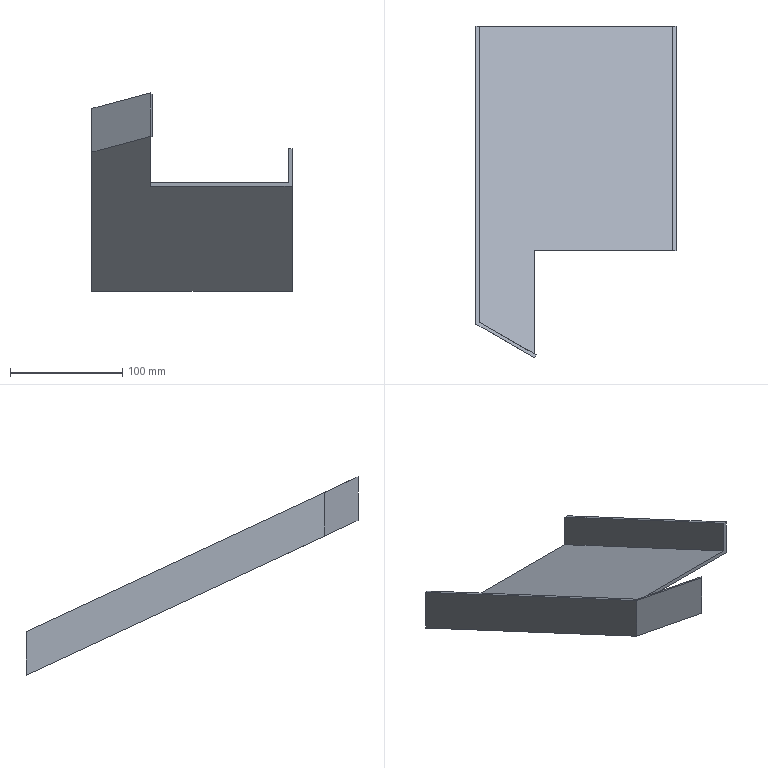Part | NX | features solid 2 | 1 solid | 15 faces | box 178 x 295.381 x 176.565 mm | volume 184168 mm3 | plane 15
STEP:
#1=CARTESIAN_POINT('',(823.,340.,-273.31));
#2=VERTEX_POINT('',#1);
#3=CARTESIAN_POINT('',(823.,340.,-270.));
#4=VERTEX_POINT('',#3);
#5=CARTESIAN_POINT('',(823.,340.,-570.));
#6=DIRECTION('',(0.,0.,1.));
#7=VECTOR('',#6,1000.);
#8=LINE('',#5,#7);
#9=EDGE_CURVE('',#2,#4,#8,.T.);
#10=ORIENTED_EDGE('',*,*,#9,.F.);
#11=CARTESIAN_POINT('',(949.,340.,-273.31));
#12=VERTEX_POINT('',#11);
#13=CARTESIAN_POINT('',(-793.,340.,-273.31));
#14=DIRECTION('',(-1.,0.,0.));
#15=VECTOR('',#14,1000.);
#16=LINE('',#13,#15);
#17=EDGE_CURVE('',#12,#2,#16,.T.);
#18=ORIENTED_EDGE('',*,*,#17,.F.);
#19=CARTESIAN_POINT('',(949.,340.,-240.));
#20=VERTEX_POINT('',#19);
#21=CARTESIAN_POINT('',(949.,340.,-270.));
#22=DIRECTION('',(0.,0.,-1.));
#23=VECTOR('',#22,1000.);
#24=LINE('',#21,#23);
#25=EDGE_CURVE('',#20,#12,#24,.T.);
#26=ORIENTED_EDGE('',*,*,#25,.F.);
#27=CARTESIAN_POINT('',(946.,340.,-240.));
#28=VERTEX_POINT('',#27);
#29=CARTESIAN_POINT('',(949.,340.,-240.));
#30=DIRECTION('',(1.,0.,0.));
#31=VECTOR('',#30,1000.);
#32=LINE('',#29,#31);
#33=EDGE_CURVE('',#20,#28,#32,.F.);
#34=ORIENTED_EDGE('',*,*,#33,.T.);
#35=CARTESIAN_POINT('',(946.,340.,-270.));
#36=VERTEX_POINT('',#35);
#37=CARTESIAN_POINT('',(946.,340.,-270.));
#38=DIRECTION('',(0.,0.,1.));
#39=VECTOR('',#38,1000.);
#40=LINE('',#37,#39);
#41=EDGE_CURVE('',#36,#28,#40,.T.);
#42=ORIENTED_EDGE('',*,*,#41,.F.);
#43=CARTESIAN_POINT('',(-793.,340.,-270.));
#44=DIRECTION('',(-1.,0.,0.));
#45=VECTOR('',#44,1000.);
#46=LINE('',#43,#45);
#47=EDGE_CURVE('',#36,#4,#46,.T.);
#48=ORIENTED_EDGE('',*,*,#47,.T.);
#49=EDGE_LOOP('',(#10,#18,#26,#34,#42,#48));
#50=FACE_BOUND('',#49,.T.);
#51=CARTESIAN_POINT('',(-793.,340.,-570.));
#52=DIRECTION('',(0.,-1.,0.));
#53=DIRECTION('',(0.,0.,-1.));
#54=AXIS2_PLACEMENT_3D('',#51,#52,#53);
#55=PLANE('',#54);
#56=ADVANCED_FACE('',(#50),#55,.T.);
#57=CARTESIAN_POINT('',(823.,248.083,-227.139));
#58=VERTEX_POINT('',#57);
#59=CARTESIAN_POINT('',(774.,276.374,-240.331));
#60=VERTEX_POINT('',#59);
#61=CARTESIAN_POINT('',(860.269,226.566,-217.105));
#62=DIRECTION('',(-0.8434,0.4869,-0.2271));
#63=VECTOR('',#62,1000.);
#64=LINE('',#61,#63);
#65=EDGE_CURVE('',#58,#60,#64,.T.);
#66=ORIENTED_EDGE('',*,*,#65,.F.);
#67=CARTESIAN_POINT('',(823.,340.,-270.));
#68=DIRECTION('',(0.,0.9063,-0.4226));
#69=VECTOR('',#68,1000.);
#70=LINE('',#67,#69);
#71=EDGE_CURVE('',#58,#4,#70,.T.);
#72=ORIENTED_EDGE('',*,*,#71,.T.);
#73=ORIENTED_EDGE('',*,*,#47,.F.);
#74=CARTESIAN_POINT('',(946.,540.,-363.262));
#75=VERTEX_POINT('',#74);
#76=CARTESIAN_POINT('',(946.,340.,-270.));
#77=DIRECTION('',(0.,0.9063,-0.4226));
#78=VECTOR('',#77,1000.);
#79=LINE('',#76,#78);
#80=EDGE_CURVE('',#36,#75,#79,.T.);
#81=ORIENTED_EDGE('',*,*,#80,.T.);
#82=CARTESIAN_POINT('',(774.,540.,-363.262));
#83=VERTEX_POINT('',#82);
#84=CARTESIAN_POINT('',(940.,540.,-363.262));
#85=DIRECTION('',(1.,0.,0.));
#86=VECTOR('',#85,1000.);
#87=LINE('',#84,#86);
#88=EDGE_CURVE('',#75,#83,#87,.F.);
#89=ORIENTED_EDGE('',*,*,#88,.T.);
#90=CARTESIAN_POINT('',(774.,340.,-270.));
#91=DIRECTION('',(0.,0.9063,-0.4226));
#92=VECTOR('',#91,1000.);
#93=LINE('',#90,#92);
#94=EDGE_CURVE('',#60,#83,#93,.T.);
#95=ORIENTED_EDGE('',*,*,#94,.F.);
#96=EDGE_LOOP('',(#66,#72,#73,#81,#89,#95));
#97=FACE_BOUND('',#96,.T.);
#98=CARTESIAN_POINT('',(940.,340.,-270.));
#99=DIRECTION('',(0.,0.4226,0.9063));
#100=DIRECTION('',(0.,-0.9063,0.4226));
#101=AXIS2_PLACEMENT_3D('',#98,#99,#100);
#102=PLANE('',#101);
#103=ADVANCED_FACE('',(#97),#102,.T.);
#104=CARTESIAN_POINT('',(949.,540.,-333.262));
#105=VERTEX_POINT('',#104);
#106=CARTESIAN_POINT('',(949.,540.,-366.572));
#107=VERTEX_POINT('',#106);
#108=CARTESIAN_POINT('',(949.,540.,-120.));
#109=DIRECTION('',(0.,0.,1.));
#110=VECTOR('',#109,1000.);
#111=LINE('',#108,#110);
#112=EDGE_CURVE('',#105,#107,#111,.F.);
#113=ORIENTED_EDGE('',*,*,#112,.F.);
#114=CARTESIAN_POINT('',(949.,340.,-240.));
#115=DIRECTION('',(0.,0.9063,-0.4226));
#116=VECTOR('',#115,1000.);
#117=LINE('',#114,#116);
#118=EDGE_CURVE('',#20,#105,#117,.T.);
#119=ORIENTED_EDGE('',*,*,#118,.F.);
#120=ORIENTED_EDGE('',*,*,#25,.T.);
#121=CARTESIAN_POINT('',(949.,338.732,-272.719));
#122=DIRECTION('',(0.,0.9063,-0.4226));
#123=VECTOR('',#122,1000.);
#124=LINE('',#121,#123);
#125=EDGE_CURVE('',#12,#107,#124,.T.);
#126=ORIENTED_EDGE('',*,*,#125,.T.);
#127=EDGE_LOOP('',(#113,#119,#120,#126));
#128=FACE_BOUND('',#127,.T.);
#129=CARTESIAN_POINT('',(949.,340.,-270.));
#130=DIRECTION('',(1.,0.,0.));
#131=DIRECTION('',(0.,0.9063,-0.4226));
#132=AXIS2_PLACEMENT_3D('',#129,#130,#131);
#133=PLANE('',#132);
#134=ADVANCED_FACE('',(#128),#133,.T.);
#135=CARTESIAN_POINT('',(823.,244.619,-228.833));
#136=VERTEX_POINT('',#135);
#137=CARTESIAN_POINT('',(771.,274.642,-242.833));
#138=VERTEX_POINT('',#137);
#139=CARTESIAN_POINT('',(857.855,224.496,-219.45));
#140=DIRECTION('',(-0.8434,0.4869,-0.2271));
#141=VECTOR('',#140,1000.);
#142=LINE('',#139,#141);
#143=EDGE_CURVE('',#136,#138,#142,.T.);
#144=ORIENTED_EDGE('',*,*,#143,.F.);
#145=CARTESIAN_POINT('',(823.,244.619,-190.006));
#146=VERTEX_POINT('',#145);
#147=CARTESIAN_POINT('',(823.,244.619,-270.));
#148=DIRECTION('',(0.,0.,-1.));
#149=VECTOR('',#148,1000.);
#150=LINE('',#147,#149);
#151=EDGE_CURVE('',#146,#136,#150,.T.);
#152=ORIENTED_EDGE('',*,*,#151,.F.);
#153=CARTESIAN_POINT('',(771.,274.642,-204.006));
#154=VERTEX_POINT('',#153);
#155=CARTESIAN_POINT('',(772.832,273.584,-203.513));
#156=DIRECTION('',(-0.8434,0.4869,-0.2271));
#157=VECTOR('',#156,1000.);
#158=LINE('',#155,#157);
#159=EDGE_CURVE('',#154,#146,#158,.F.);
#160=ORIENTED_EDGE('',*,*,#159,.F.);
#161=CARTESIAN_POINT('',(771.,274.642,-240.));
#162=DIRECTION('',(0.,0.,1.));
#163=VECTOR('',#162,1000.);
#164=LINE('',#161,#163);
#165=EDGE_CURVE('',#154,#138,#164,.F.);
#166=ORIENTED_EDGE('',*,*,#165,.T.);
#167=EDGE_LOOP('',(#144,#152,#160,#166));
#168=FACE_BOUND('',#167,.T.);
#169=CARTESIAN_POINT('',(862.005,222.1,-240.));
#170=DIRECTION('',(-0.5,-0.866,0.));
#171=DIRECTION('',(-0.866,0.5,0.));
#172=AXIS2_PLACEMENT_3D('',#169,#170,#171);
#173=PLANE('',#172);
#174=ADVANCED_FACE('',(#168),#173,.T.);
#175=ORIENTED_EDGE('',*,*,#165,.F.);
#176=CARTESIAN_POINT('',(771.,540.,-327.745));
#177=VERTEX_POINT('',#176);
#178=CARTESIAN_POINT('',(771.,353.604,-240.827));
#179=DIRECTION('',(0.,0.9063,-0.4226));
#180=VECTOR('',#179,1000.);
#181=LINE('',#178,#180);
#182=EDGE_CURVE('',#154,#177,#181,.T.);
#183=ORIENTED_EDGE('',*,*,#182,.T.);
#184=CARTESIAN_POINT('',(771.,540.,-366.572));
#185=VERTEX_POINT('',#184);
#186=CARTESIAN_POINT('',(771.,540.,-270.));
#187=DIRECTION('',(0.,0.,-1.));
#188=VECTOR('',#187,1000.);
#189=LINE('',#186,#188);
#190=EDGE_CURVE('',#177,#185,#189,.T.);
#191=ORIENTED_EDGE('',*,*,#190,.T.);
#192=CARTESIAN_POINT('',(771.,338.732,-272.719));
#193=DIRECTION('',(0.,-0.9063,0.4226));
#194=VECTOR('',#193,1000.);
#195=LINE('',#192,#194);
#196=EDGE_CURVE('',#138,#185,#195,.F.);
#197=ORIENTED_EDGE('',*,*,#196,.F.);
#198=EDGE_LOOP('',(#175,#183,#191,#197));
#199=FACE_BOUND('',#198,.T.);
#200=CARTESIAN_POINT('',(771.,340.,-270.));
#201=DIRECTION('',(1.,0.,0.));
#202=DIRECTION('',(0.,0.9063,-0.4226));
#203=AXIS2_PLACEMENT_3D('',#200,#201,#202);
#204=PLANE('',#203);
#205=ADVANCED_FACE('',(#199),#204,.F.);
#206=ORIENTED_EDGE('',*,*,#17,.T.);
#207=CARTESIAN_POINT('',(823.,338.732,-272.719));
#208=DIRECTION('',(0.,0.9063,-0.4226));
#209=VECTOR('',#208,1000.);
#210=LINE('',#207,#209);
#211=EDGE_CURVE('',#136,#2,#210,.T.);
#212=ORIENTED_EDGE('',*,*,#211,.F.);
#213=ORIENTED_EDGE('',*,*,#143,.T.);
#214=ORIENTED_EDGE('',*,*,#196,.T.);
#215=CARTESIAN_POINT('',(940.,540.,-366.572));
#216=DIRECTION('',(1.,0.,0.));
#217=VECTOR('',#216,1000.);
#218=LINE('',#215,#217);
#219=EDGE_CURVE('',#107,#185,#218,.F.);
#220=ORIENTED_EDGE('',*,*,#219,.F.);
#221=ORIENTED_EDGE('',*,*,#125,.F.);
#222=EDGE_LOOP('',(#206,#212,#213,#214,#220,#221));
#223=FACE_BOUND('',#222,.T.);
#224=CARTESIAN_POINT('',(940.,338.732,-272.719));
#225=DIRECTION('',(0.,0.4226,0.9063));
#226=DIRECTION('',(0.,-0.9063,0.4226));
#227=AXIS2_PLACEMENT_3D('',#224,#225,#226);
#228=PLANE('',#227);
#229=ADVANCED_FACE('',(#223),#228,.F.);
#230=ORIENTED_EDGE('',*,*,#88,.F.);
#231=CARTESIAN_POINT('',(946.,540.,-333.262));
#232=VERTEX_POINT('',#231);
#233=CARTESIAN_POINT('',(946.,540.,-270.));
#234=DIRECTION('',(0.,0.,-1.));
#235=VECTOR('',#234,1000.);
#236=LINE('',#233,#235);
#237=EDGE_CURVE('',#75,#232,#236,.F.);
#238=ORIENTED_EDGE('',*,*,#237,.T.);
#239=CARTESIAN_POINT('',(1125.,540.,-333.262));
#240=DIRECTION('',(1.,0.,0.));
#241=VECTOR('',#240,1000.);
#242=LINE('',#239,#241);
#243=EDGE_CURVE('',#105,#232,#242,.F.);
#244=ORIENTED_EDGE('',*,*,#243,.F.);
#245=ORIENTED_EDGE('',*,*,#112,.T.);
#246=ORIENTED_EDGE('',*,*,#219,.T.);
#247=ORIENTED_EDGE('',*,*,#190,.F.);
#248=CARTESIAN_POINT('',(774.,540.,-327.745));
#249=VERTEX_POINT('',#248);
#250=CARTESIAN_POINT('',(1125.,540.,-327.745));
#251=DIRECTION('',(1.,0.,0.));
#252=VECTOR('',#251,1000.);
#253=LINE('',#250,#252);
#254=EDGE_CURVE('',#177,#249,#253,.T.);
#255=ORIENTED_EDGE('',*,*,#254,.T.);
#256=CARTESIAN_POINT('',(774.,540.,-270.));
#257=DIRECTION('',(0.,0.,-1.));
#258=VECTOR('',#257,1000.);
#259=LINE('',#256,#258);
#260=EDGE_CURVE('',#83,#249,#259,.F.);
#261=ORIENTED_EDGE('',*,*,#260,.F.);
#262=EDGE_LOOP('',(#230,#238,#244,#245,#246,#247,#255,#261));
#263=FACE_BOUND('',#262,.T.);
#264=CARTESIAN_POINT('',(1125.,540.,-120.));
#265=DIRECTION('',(0.,-1.,0.));
#266=DIRECTION('',(-1.,0.,0.));
#267=AXIS2_PLACEMENT_3D('',#264,#265,#266);
#268=PLANE('',#267);
#269=ADVANCED_FACE('',(#263),#268,.F.);
#270=ORIENTED_EDGE('',*,*,#243,.T.);
#271=CARTESIAN_POINT('',(946.,340.,-240.));
#272=DIRECTION('',(0.,0.9063,-0.4226));
#273=VECTOR('',#272,1000.);
#274=LINE('',#271,#273);
#275=EDGE_CURVE('',#28,#232,#274,.T.);
#276=ORIENTED_EDGE('',*,*,#275,.F.);
#277=ORIENTED_EDGE('',*,*,#33,.F.);
#278=ORIENTED_EDGE('',*,*,#118,.T.);
#279=EDGE_LOOP('',(#270,#276,#277,#278));
#280=FACE_BOUND('',#279,.T.);
#281=CARTESIAN_POINT('',(949.,340.,-240.));
#282=DIRECTION('',(0.,-0.4226,-0.9063));
#283=DIRECTION('',(0.,0.9063,-0.4226));
#284=AXIS2_PLACEMENT_3D('',#281,#282,#283);
#285=PLANE('',#284);
#286=ADVANCED_FACE('',(#280),#285,.F.);
#287=ORIENTED_EDGE('',*,*,#275,.T.);
#288=ORIENTED_EDGE('',*,*,#237,.F.);
#289=ORIENTED_EDGE('',*,*,#80,.F.);
#290=ORIENTED_EDGE('',*,*,#41,.T.);
#291=EDGE_LOOP('',(#287,#288,#289,#290));
#292=FACE_BOUND('',#291,.T.);
#293=CARTESIAN_POINT('',(946.,340.,-270.));
#294=DIRECTION('',(1.,0.,0.));
#295=DIRECTION('',(0.,1.,0.));
#296=AXIS2_PLACEMENT_3D('',#293,#294,#295);
#297=PLANE('',#296);
#298=ADVANCED_FACE('',(#292),#297,.F.);
#299=ORIENTED_EDGE('',*,*,#182,.F.);
#300=ORIENTED_EDGE('',*,*,#159,.T.);
#301=CARTESIAN_POINT('',(824.5,247.217,-191.218));
#302=VERTEX_POINT('',#301);
#303=CARTESIAN_POINT('',(866.759,320.413,-225.349));
#304=DIRECTION('',(0.4636,0.803,-0.3745));
#305=VECTOR('',#304,1000.);
#306=LINE('',#303,#305);
#307=EDGE_CURVE('',#146,#302,#306,.T.);
#308=ORIENTED_EDGE('',*,*,#307,.T.);
#309=CARTESIAN_POINT('',(774.,276.374,-204.814));
#310=VERTEX_POINT('',#309);
#311=CARTESIAN_POINT('',(774.564,276.048,-204.662));
#312=DIRECTION('',(0.8434,-0.4869,0.2271));
#313=VECTOR('',#312,1000.);
#314=LINE('',#311,#313);
#315=EDGE_CURVE('',#302,#310,#314,.F.);
#316=ORIENTED_EDGE('',*,*,#315,.T.);
#317=CARTESIAN_POINT('',(774.,342.113,-235.468));
#318=DIRECTION('',(0.,-0.9063,0.4226));
#319=VECTOR('',#318,1000.);
#320=LINE('',#317,#319);
#321=EDGE_CURVE('',#310,#249,#320,.F.);
#322=ORIENTED_EDGE('',*,*,#321,.T.);
#323=ORIENTED_EDGE('',*,*,#254,.F.);
#324=EDGE_LOOP('',(#299,#300,#308,#316,#322,#323));
#325=FACE_BOUND('',#324,.T.);
#326=CARTESIAN_POINT('',(821.,342.113,-235.468));
#327=DIRECTION('',(0.,-0.4226,-0.9063));
#328=DIRECTION('',(0.,0.9063,-0.4226));
#329=AXIS2_PLACEMENT_3D('',#326,#327,#328);
#330=PLANE('',#329);
#331=ADVANCED_FACE('',(#325),#330,.F.);
#332=CARTESIAN_POINT('',(774.,276.374,-270.));
#333=DIRECTION('',(0.,0.,1.));
#334=VECTOR('',#333,1000.);
#335=LINE('',#332,#334);
#336=EDGE_CURVE('',#60,#310,#335,.T.);
#337=ORIENTED_EDGE('',*,*,#336,.F.);
#338=ORIENTED_EDGE('',*,*,#94,.T.);
#339=ORIENTED_EDGE('',*,*,#260,.T.);
#340=ORIENTED_EDGE('',*,*,#321,.F.);
#341=EDGE_LOOP('',(#337,#338,#339,#340));
#342=FACE_BOUND('',#341,.T.);
#343=CARTESIAN_POINT('',(774.,340.,-270.));
#344=DIRECTION('',(1.,0.,0.));
#345=DIRECTION('',(0.,1.,0.));
#346=AXIS2_PLACEMENT_3D('',#343,#344,#345);
#347=PLANE('',#346);
#348=ADVANCED_FACE('',(#342),#347,.T.);
#349=CARTESIAN_POINT('',(823.,248.083,-229.237));
#350=VERTEX_POINT('',#349);
#351=CARTESIAN_POINT('',(823.,343.456,-240.355));
#352=DIRECTION('',(0.,0.9933,-0.1158));
#353=VECTOR('',#352,1000.);
#354=LINE('',#351,#353);
#355=EDGE_CURVE('',#136,#350,#354,.T.);
#356=ORIENTED_EDGE('',*,*,#355,.F.);
#357=ORIENTED_EDGE('',*,*,#211,.T.);
#358=ORIENTED_EDGE('',*,*,#9,.T.);
#359=ORIENTED_EDGE('',*,*,#71,.F.);
#360=CARTESIAN_POINT('',(823.,248.083,-270.));
#361=DIRECTION('',(0.,0.,1.));
#362=VECTOR('',#361,1000.);
#363=LINE('',#360,#362);
#364=EDGE_CURVE('',#350,#58,#363,.T.);
#365=ORIENTED_EDGE('',*,*,#364,.F.);
#366=EDGE_LOOP('',(#356,#357,#358,#359,#365));
#367=FACE_BOUND('',#366,.T.);
#368=CARTESIAN_POINT('',(823.,340.,-270.));
#369=DIRECTION('',(1.,0.,0.));
#370=DIRECTION('',(0.,1.,0.));
#371=AXIS2_PLACEMENT_3D('',#368,#369,#370);
#372=PLANE('',#371);
#373=ADVANCED_FACE('',(#367),#372,.T.);
#374=CARTESIAN_POINT('',(824.5,247.217,-228.833));
#375=VERTEX_POINT('',#374);
#376=CARTESIAN_POINT('',(823.,244.619,-228.833));
#377=DIRECTION('',(0.5,0.866,0.));
#378=VECTOR('',#377,1000.);
#379=LINE('',#376,#378);
#380=EDGE_CURVE('',#136,#375,#379,.T.);
#381=ORIENTED_EDGE('',*,*,#380,.F.);
#382=ORIENTED_EDGE('',*,*,#355,.T.);
#383=CARTESIAN_POINT('',(824.5,247.217,-228.833));
#384=DIRECTION('',(-0.8434,0.4869,-0.2271));
#385=VECTOR('',#384,1000.);
#386=LINE('',#383,#385);
#387=EDGE_CURVE('',#375,#350,#386,.T.);
#388=ORIENTED_EDGE('',*,*,#387,.F.);
#389=EDGE_LOOP('',(#381,#382,#388));
#390=FACE_BOUND('',#389,.T.);
#391=CARTESIAN_POINT('',(823.,244.619,-228.833));
#392=DIRECTION('',(0.1966,-0.1135,-0.9739));
#393=DIRECTION('',(-0.8434,0.4869,-0.2271));
#394=AXIS2_PLACEMENT_3D('',#391,#392,#393);
#395=PLANE('',#394);
#396=ADVANCED_FACE('',(#390),#395,.T.);
#397=ORIENTED_EDGE('',*,*,#65,.T.);
#398=ORIENTED_EDGE('',*,*,#336,.T.);
#399=ORIENTED_EDGE('',*,*,#315,.F.);
#400=CARTESIAN_POINT('',(824.5,247.217,-228.833));
#401=DIRECTION('',(0.,0.,1.));
#402=VECTOR('',#401,1000.);
#403=LINE('',#400,#402);
#404=EDGE_CURVE('',#375,#302,#403,.T.);
#405=ORIENTED_EDGE('',*,*,#404,.F.);
#406=ORIENTED_EDGE('',*,*,#387,.T.);
#407=ORIENTED_EDGE('',*,*,#364,.T.);
#408=EDGE_LOOP('',(#397,#398,#399,#405,#406,#407));
#409=FACE_BOUND('',#408,.T.);
#410=CARTESIAN_POINT('',(824.5,247.217,-228.833));
#411=DIRECTION('',(0.5,0.866,0.));
#412=DIRECTION('',(-0.866,0.5,0.));
#413=AXIS2_PLACEMENT_3D('',#410,#411,#412);
#414=PLANE('',#413);
#415=ADVANCED_FACE('',(#409),#414,.T.);
#416=ORIENTED_EDGE('',*,*,#151,.T.);
#417=ORIENTED_EDGE('',*,*,#380,.T.);
#418=ORIENTED_EDGE('',*,*,#404,.T.);
#419=ORIENTED_EDGE('',*,*,#307,.F.);
#420=EDGE_LOOP('',(#416,#417,#418,#419));
#421=FACE_BOUND('',#420,.T.);
#422=CARTESIAN_POINT('',(823.,244.619,-228.833));
#423=DIRECTION('',(-0.866,0.5,0.));
#424=DIRECTION('',(0.,0.,1.));
#425=AXIS2_PLACEMENT_3D('',#422,#423,#424);
#426=PLANE('',#425);
#427=ADVANCED_FACE('',(#421),#426,.F.);
#428=CLOSED_SHELL('',(#56,#103,#134,#174,#205,#229,#269,#286,#298,#331,#348,#373,#396,#415,#427));
#429=MANIFOLD_SOLID_BREP('',#428);
#430=(LENGTH_UNIT()NAMED_UNIT(*)SI_UNIT(.MILLI.,.METRE.));
#431=UNCERTAINTY_MEASURE_WITH_UNIT(LENGTH_MEASURE(0.00001),#430,'','');
#432=(NAMED_UNIT(*)PLANE_ANGLE_UNIT()SI_UNIT($,.RADIAN.));
#433=(NAMED_UNIT(*)SI_UNIT($,.STERADIAN.)SOLID_ANGLE_UNIT());
#434=(GEOMETRIC_REPRESENTATION_CONTEXT(3)GLOBAL_UNCERTAINTY_ASSIGNED_CONTEXT((#431))GLOBAL_UNIT_ASSIGNED_CONTEXT((#430,#432,#433))REPRESENTATION_CONTEXT('',''));
#435=ADVANCED_BREP_SHAPE_REPRESENTATION('',(#429),#434);